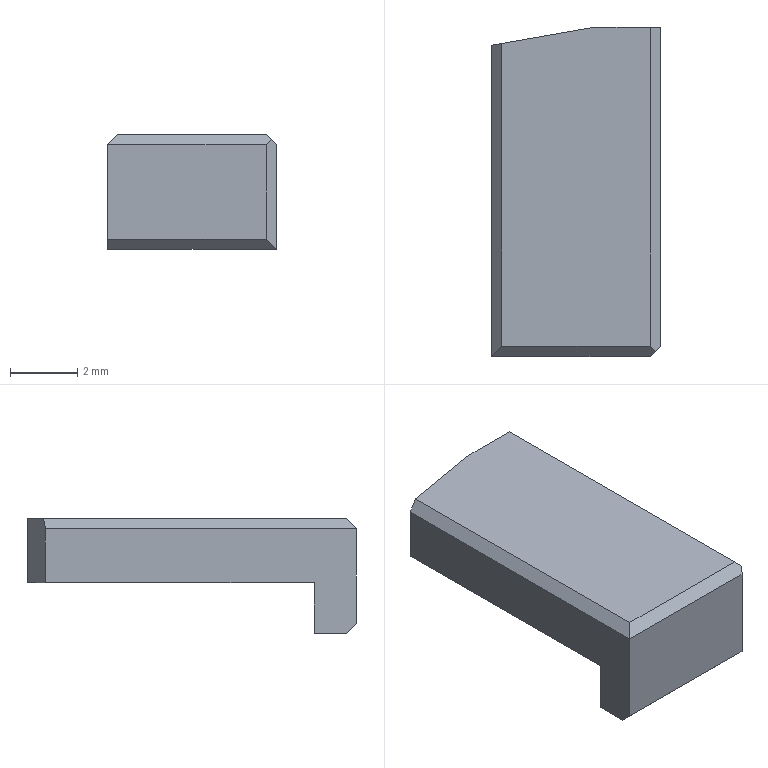Part | NX | 1 solid | 14 faces | box 5 x 9.75 x 3.4 mm | volume 99.073 mm3 | plane 14
STEP:
#1=CARTESIAN_POINT('',(-20.11,-56.129,7.853));
#2=VERTEX_POINT('',#1);
#3=CARTESIAN_POINT('',(-20.11,-64.629,7.853));
#4=VERTEX_POINT('',#3);
#5=CARTESIAN_POINT('',(-20.11,-63.129,7.853));
#6=DIRECTION('',(0.,-1.,0.));
#7=VECTOR('',#6,1000.);
#8=LINE('',#5,#7);
#9=EDGE_CURVE('',#2,#4,#8,.T.);
#10=ORIENTED_EDGE('',*,*,#9,.T.);
#11=CARTESIAN_POINT('',(-25.11,-64.629,7.853));
#12=VERTEX_POINT('',#11);
#13=CARTESIAN_POINT('',(-22.513,-64.629,7.853));
#14=DIRECTION('',(1.,0.,0.));
#15=VECTOR('',#14,1000.);
#16=LINE('',#13,#15);
#17=EDGE_CURVE('',#12,#4,#16,.T.);
#18=ORIENTED_EDGE('',*,*,#17,.F.);
#19=CARTESIAN_POINT('',(-25.11,-56.658,7.853));
#20=VERTEX_POINT('',#19);
#21=CARTESIAN_POINT('',(-25.11,-63.129,7.853));
#22=DIRECTION('',(0.,1.,0.));
#23=VECTOR('',#22,1000.);
#24=LINE('',#21,#23);
#25=EDGE_CURVE('',#12,#20,#24,.T.);
#26=ORIENTED_EDGE('',*,*,#25,.T.);
#27=CARTESIAN_POINT('',(-22.11,-56.129,7.853));
#28=VERTEX_POINT('',#27);
#29=CARTESIAN_POINT('',(-22.513,-56.2,7.853));
#30=DIRECTION('',(0.9848,0.1736,0.));
#31=VECTOR('',#30,1000.);
#32=LINE('',#29,#31);
#33=EDGE_CURVE('',#20,#28,#32,.T.);
#34=ORIENTED_EDGE('',*,*,#33,.T.);
#35=CARTESIAN_POINT('',(-22.513,-56.129,7.853));
#36=DIRECTION('',(1.,0.,0.));
#37=VECTOR('',#36,1000.);
#38=LINE('',#35,#37);
#39=EDGE_CURVE('',#28,#2,#38,.T.);
#40=ORIENTED_EDGE('',*,*,#39,.T.);
#41=EDGE_LOOP('',(#10,#18,#26,#34,#40));
#42=FACE_BOUND('',#41,.T.);
#43=CARTESIAN_POINT('',(-32.11,-63.129,7.853));
#44=DIRECTION('',(0.,0.,-1.));
#45=DIRECTION('',(0.,-1.,0.));
#46=AXIS2_PLACEMENT_3D('',#43,#44,#45);
#47=PLANE('',#46);
#48=ADVANCED_FACE('',(#42),#47,.T.);
#49=CARTESIAN_POINT('',(-25.11,-56.658,9.453));
#50=VERTEX_POINT('',#49);
#51=CARTESIAN_POINT('',(-25.11,-65.879,9.453));
#52=VERTEX_POINT('',#51);
#53=CARTESIAN_POINT('',(-25.11,-61.268,9.453));
#54=DIRECTION('',(0.,-1.,0.));
#55=VECTOR('',#54,1000.);
#56=LINE('',#53,#55);
#57=EDGE_CURVE('',#50,#52,#56,.T.);
#58=ORIENTED_EDGE('',*,*,#57,.F.);
#59=CARTESIAN_POINT('',(-25.11,-56.658,8.803));
#60=DIRECTION('',(0.,0.,-1.));
#61=VECTOR('',#60,1000.);
#62=LINE('',#59,#61);
#63=EDGE_CURVE('',#50,#20,#62,.T.);
#64=ORIENTED_EDGE('',*,*,#63,.T.);
#65=ORIENTED_EDGE('',*,*,#25,.F.);
#66=CARTESIAN_POINT('',(-25.11,-64.629,6.353));
#67=VERTEX_POINT('',#66);
#68=CARTESIAN_POINT('',(-25.11,-64.629,13.966));
#69=DIRECTION('',(0.,0.,-1.));
#70=VECTOR('',#69,1000.);
#71=LINE('',#68,#70);
#72=EDGE_CURVE('',#12,#67,#71,.T.);
#73=ORIENTED_EDGE('',*,*,#72,.T.);
#74=CARTESIAN_POINT('',(-25.11,-65.579,6.353));
#75=VERTEX_POINT('',#74);
#76=CARTESIAN_POINT('',(-25.11,-63.129,6.353));
#77=DIRECTION('',(0.,1.,0.));
#78=VECTOR('',#77,1000.);
#79=LINE('',#76,#78);
#80=EDGE_CURVE('',#75,#67,#79,.T.);
#81=ORIENTED_EDGE('',*,*,#80,.F.);
#82=CARTESIAN_POINT('',(-25.11,-65.879,6.653));
#83=VERTEX_POINT('',#82);
#84=CARTESIAN_POINT('',(-25.11,-63.129,3.903));
#85=DIRECTION('',(0.,0.7071,-0.7071));
#86=VECTOR('',#85,1000.);
#87=LINE('',#84,#86);
#88=EDGE_CURVE('',#83,#75,#87,.T.);
#89=ORIENTED_EDGE('',*,*,#88,.F.);
#90=CARTESIAN_POINT('',(-25.11,-65.879,13.966));
#91=DIRECTION('',(0.,0.,1.));
#92=VECTOR('',#91,1000.);
#93=LINE('',#90,#92);
#94=EDGE_CURVE('',#83,#52,#93,.T.);
#95=ORIENTED_EDGE('',*,*,#94,.T.);
#96=EDGE_LOOP('',(#58,#64,#65,#73,#81,#89,#95));
#97=FACE_BOUND('',#96,.T.);
#98=CARTESIAN_POINT('',(-25.11,-63.129,9.253));
#99=DIRECTION('',(-1.,0.,0.));
#100=DIRECTION('',(0.,0.,1.));
#101=AXIS2_PLACEMENT_3D('',#98,#99,#100);
#102=PLANE('',#101);
#103=ADVANCED_FACE('',(#97),#102,.T.);
#104=CARTESIAN_POINT('',(-20.41,-65.579,9.753));
#105=VERTEX_POINT('',#104);
#106=CARTESIAN_POINT('',(-20.41,-56.129,9.753));
#107=VERTEX_POINT('',#106);
#108=CARTESIAN_POINT('',(-20.41,-61.004,9.753));
#109=DIRECTION('',(0.,1.,0.));
#110=VECTOR('',#109,1000.);
#111=LINE('',#108,#110);
#112=EDGE_CURVE('',#105,#107,#111,.T.);
#113=ORIENTED_EDGE('',*,*,#112,.T.);
#114=CARTESIAN_POINT('',(-22.11,-56.129,9.753));
#115=VERTEX_POINT('',#114);
#116=CARTESIAN_POINT('',(-22.513,-56.129,9.753));
#117=DIRECTION('',(-1.,0.,0.));
#118=VECTOR('',#117,1000.);
#119=LINE('',#116,#118);
#120=EDGE_CURVE('',#107,#115,#119,.T.);
#121=ORIENTED_EDGE('',*,*,#120,.T.);
#122=CARTESIAN_POINT('',(-24.81,-56.605,9.753));
#123=VERTEX_POINT('',#122);
#124=CARTESIAN_POINT('',(-22.513,-56.2,9.753));
#125=DIRECTION('',(-0.9848,-0.1736,0.));
#126=VECTOR('',#125,1000.);
#127=LINE('',#124,#126);
#128=EDGE_CURVE('',#115,#123,#127,.T.);
#129=ORIENTED_EDGE('',*,*,#128,.T.);
#130=CARTESIAN_POINT('',(-24.81,-65.579,9.753));
#131=VERTEX_POINT('',#130);
#132=CARTESIAN_POINT('',(-24.81,-61.268,9.753));
#133=DIRECTION('',(0.,-1.,0.));
#134=VECTOR('',#133,1000.);
#135=LINE('',#132,#134);
#136=EDGE_CURVE('',#123,#131,#135,.T.);
#137=ORIENTED_EDGE('',*,*,#136,.T.);
#138=CARTESIAN_POINT('',(-22.61,-65.579,9.753));
#139=DIRECTION('',(1.,0.,0.));
#140=VECTOR('',#139,1000.);
#141=LINE('',#138,#140);
#142=EDGE_CURVE('',#131,#105,#141,.T.);
#143=ORIENTED_EDGE('',*,*,#142,.T.);
#144=EDGE_LOOP('',(#113,#121,#129,#137,#143));
#145=FACE_BOUND('',#144,.T.);
#146=CARTESIAN_POINT('',(-16.11,-63.129,9.753));
#147=DIRECTION('',(0.,0.,1.));
#148=DIRECTION('',(1.,0.,0.));
#149=AXIS2_PLACEMENT_3D('',#146,#147,#148);
#150=PLANE('',#149);
#151=ADVANCED_FACE('',(#145),#150,.T.);
#152=CARTESIAN_POINT('',(-20.11,-56.129,9.453));
#153=VERTEX_POINT('',#152);
#154=CARTESIAN_POINT('',(-20.11,-56.129,13.966));
#155=DIRECTION('',(0.,0.,1.));
#156=VECTOR('',#155,1000.);
#157=LINE('',#154,#156);
#158=EDGE_CURVE('',#2,#153,#157,.T.);
#159=ORIENTED_EDGE('',*,*,#158,.T.);
#160=CARTESIAN_POINT('',(-20.11,-65.579,9.453));
#161=VERTEX_POINT('',#160);
#162=CARTESIAN_POINT('',(-20.11,-61.004,9.453));
#163=DIRECTION('',(0.,1.,0.));
#164=VECTOR('',#163,1000.);
#165=LINE('',#162,#164);
#166=EDGE_CURVE('',#161,#153,#165,.T.);
#167=ORIENTED_EDGE('',*,*,#166,.F.);
#168=CARTESIAN_POINT('',(-20.11,-65.579,6.353));
#169=VERTEX_POINT('',#168);
#170=CARTESIAN_POINT('',(-20.11,-65.579,8.053));
#171=DIRECTION('',(0.,0.,1.));
#172=VECTOR('',#171,1000.);
#173=LINE('',#170,#172);
#174=EDGE_CURVE('',#169,#161,#173,.T.);
#175=ORIENTED_EDGE('',*,*,#174,.F.);
#176=CARTESIAN_POINT('',(-20.11,-64.629,6.353));
#177=VERTEX_POINT('',#176);
#178=CARTESIAN_POINT('',(-20.11,-63.129,6.353));
#179=DIRECTION('',(0.,-1.,0.));
#180=VECTOR('',#179,1000.);
#181=LINE('',#178,#180);
#182=EDGE_CURVE('',#177,#169,#181,.T.);
#183=ORIENTED_EDGE('',*,*,#182,.F.);
#184=CARTESIAN_POINT('',(-20.11,-64.629,13.966));
#185=DIRECTION('',(0.,0.,-1.));
#186=VECTOR('',#185,1000.);
#187=LINE('',#184,#186);
#188=EDGE_CURVE('',#4,#177,#187,.T.);
#189=ORIENTED_EDGE('',*,*,#188,.F.);
#190=ORIENTED_EDGE('',*,*,#9,.F.);
#191=EDGE_LOOP('',(#159,#167,#175,#183,#189,#190));
#192=FACE_BOUND('',#191,.T.);
#193=CARTESIAN_POINT('',(-20.11,-63.129,7.853));
#194=DIRECTION('',(1.,0.,0.));
#195=DIRECTION('',(0.,-1.,0.));
#196=AXIS2_PLACEMENT_3D('',#193,#194,#195);
#197=PLANE('',#196);
#198=ADVANCED_FACE('',(#192),#197,.T.);
#199=CARTESIAN_POINT('',(-22.61,-65.579,6.353));
#200=DIRECTION('',(-1.,0.,0.));
#201=VECTOR('',#200,1000.);
#202=LINE('',#199,#201);
#203=EDGE_CURVE('',#169,#75,#202,.T.);
#204=ORIENTED_EDGE('',*,*,#203,.T.);
#205=ORIENTED_EDGE('',*,*,#80,.T.);
#206=CARTESIAN_POINT('',(-22.513,-64.629,6.353));
#207=DIRECTION('',(1.,0.,0.));
#208=VECTOR('',#207,1000.);
#209=LINE('',#206,#208);
#210=EDGE_CURVE('',#67,#177,#209,.T.);
#211=ORIENTED_EDGE('',*,*,#210,.T.);
#212=ORIENTED_EDGE('',*,*,#182,.T.);
#213=EDGE_LOOP('',(#204,#205,#211,#212));
#214=FACE_BOUND('',#213,.T.);
#215=CARTESIAN_POINT('',(-19.282,-63.809,6.353));
#216=DIRECTION('',(0.,0.,-1.));
#217=DIRECTION('',(0.,-1.,0.));
#218=AXIS2_PLACEMENT_3D('',#215,#216,#217);
#219=PLANE('',#218);
#220=ADVANCED_FACE('',(#214),#219,.T.);
#221=ORIENTED_EDGE('',*,*,#57,.T.);
#222=CARTESIAN_POINT('',(-22.513,-63.282,12.05));
#223=DIRECTION('',(0.5774,0.5774,0.5774));
#224=VECTOR('',#223,1000.);
#225=LINE('',#222,#224);
#226=EDGE_CURVE('',#52,#131,#225,.T.);
#227=ORIENTED_EDGE('',*,*,#226,.T.);
#228=ORIENTED_EDGE('',*,*,#136,.F.);
#229=CARTESIAN_POINT('',(-22.513,-56.2,12.05));
#230=DIRECTION('',(-0.7017,-0.1237,-0.7017));
#231=VECTOR('',#230,1000.);
#232=LINE('',#229,#231);
#233=EDGE_CURVE('',#123,#50,#232,.T.);
#234=ORIENTED_EDGE('',*,*,#233,.T.);
#235=EDGE_LOOP('',(#221,#227,#228,#234));
#236=FACE_BOUND('',#235,.T.);
#237=CARTESIAN_POINT('',(-24.96,-61.268,9.603));
#238=DIRECTION('',(0.7071,0.,-0.7071));
#239=DIRECTION('',(0.,-1.,0.));
#240=AXIS2_PLACEMENT_3D('',#237,#238,#239);
#241=PLANE('',#240);
#242=ADVANCED_FACE('',(#236),#241,.F.);
#243=ORIENTED_EDGE('',*,*,#112,.F.);
#244=CARTESIAN_POINT('',(-20.26,-65.729,9.603));
#245=VERTEX_POINT('',#244);
#246=CARTESIAN_POINT('',(-22.86,-63.129,12.203));
#247=DIRECTION('',(-0.5774,0.5774,0.5774));
#248=VECTOR('',#247,1000.);
#249=LINE('',#246,#248);
#250=EDGE_CURVE('',#245,#105,#249,.T.);
#251=ORIENTED_EDGE('',*,*,#250,.F.);
#252=CARTESIAN_POINT('',(-17.66,-63.129,7.003));
#253=DIRECTION('',(0.5774,0.5774,-0.5774));
#254=VECTOR('',#253,1000.);
#255=LINE('',#252,#254);
#256=EDGE_CURVE('',#245,#161,#255,.T.);
#257=ORIENTED_EDGE('',*,*,#256,.T.);
#258=ORIENTED_EDGE('',*,*,#166,.T.);
#259=CARTESIAN_POINT('',(-24.624,-56.129,13.966));
#260=DIRECTION('',(0.7071,0.,-0.7071));
#261=VECTOR('',#260,1000.);
#262=LINE('',#259,#261);
#263=EDGE_CURVE('',#107,#153,#262,.T.);
#264=ORIENTED_EDGE('',*,*,#263,.F.);
#265=EDGE_LOOP('',(#243,#251,#257,#258,#264));
#266=FACE_BOUND('',#265,.T.);
#267=CARTESIAN_POINT('',(-20.26,-61.004,9.603));
#268=DIRECTION('',(0.7071,0.,0.7071));
#269=DIRECTION('',(0.,-1.,0.));
#270=AXIS2_PLACEMENT_3D('',#267,#268,#269);
#271=PLANE('',#270);
#272=ADVANCED_FACE('',(#266),#271,.T.);
#273=ORIENTED_EDGE('',*,*,#203,.F.);
#274=CARTESIAN_POINT('',(-20.41,-65.879,6.653));
#275=VERTEX_POINT('',#274);
#276=CARTESIAN_POINT('',(-17.66,-63.129,3.903));
#277=DIRECTION('',(0.5774,0.5774,-0.5774));
#278=VECTOR('',#277,1000.);
#279=LINE('',#276,#278);
#280=EDGE_CURVE('',#275,#169,#279,.T.);
#281=ORIENTED_EDGE('',*,*,#280,.F.);
#282=CARTESIAN_POINT('',(-22.61,-65.879,6.653));
#283=DIRECTION('',(-1.,0.,0.));
#284=VECTOR('',#283,1000.);
#285=LINE('',#282,#284);
#286=EDGE_CURVE('',#275,#83,#285,.T.);
#287=ORIENTED_EDGE('',*,*,#286,.T.);
#288=ORIENTED_EDGE('',*,*,#88,.T.);
#289=EDGE_LOOP('',(#273,#281,#287,#288));
#290=FACE_BOUND('',#289,.T.);
#291=CARTESIAN_POINT('',(-22.61,-65.729,6.503));
#292=DIRECTION('',(0.,-0.7071,-0.7071));
#293=DIRECTION('',(0.,-0.7071,0.7071));
#294=AXIS2_PLACEMENT_3D('',#291,#292,#293);
#295=PLANE('',#294);
#296=ADVANCED_FACE('',(#290),#295,.T.);
#297=CARTESIAN_POINT('',(-22.11,-56.129,8.803));
#298=DIRECTION('',(0.,0.,-1.));
#299=VECTOR('',#298,1000.);
#300=LINE('',#297,#299);
#301=EDGE_CURVE('',#115,#28,#300,.T.);
#302=ORIENTED_EDGE('',*,*,#301,.F.);
#303=ORIENTED_EDGE('',*,*,#120,.F.);
#304=ORIENTED_EDGE('',*,*,#263,.T.);
#305=ORIENTED_EDGE('',*,*,#158,.F.);
#306=ORIENTED_EDGE('',*,*,#39,.F.);
#307=EDGE_LOOP('',(#302,#303,#304,#305,#306));
#308=FACE_BOUND('',#307,.T.);
#309=CARTESIAN_POINT('',(-22.513,-56.129,13.966));
#310=DIRECTION('',(0.,-1.,0.));
#311=DIRECTION('',(-1.,0.,0.));
#312=AXIS2_PLACEMENT_3D('',#309,#310,#311);
#313=PLANE('',#312);
#314=ADVANCED_FACE('',(#308),#313,.F.);
#315=ORIENTED_EDGE('',*,*,#301,.T.);
#316=ORIENTED_EDGE('',*,*,#33,.F.);
#317=ORIENTED_EDGE('',*,*,#63,.F.);
#318=ORIENTED_EDGE('',*,*,#233,.F.);
#319=ORIENTED_EDGE('',*,*,#128,.F.);
#320=EDGE_LOOP('',(#315,#316,#317,#318,#319));
#321=FACE_BOUND('',#320,.T.);
#322=CARTESIAN_POINT('',(-23.61,-56.393,8.803));
#323=DIRECTION('',(0.1736,-0.9848,0.));
#324=DIRECTION('',(0.,0.,-1.));
#325=AXIS2_PLACEMENT_3D('',#322,#323,#324);
#326=PLANE('',#325);
#327=ADVANCED_FACE('',(#321),#326,.F.);
#328=CARTESIAN_POINT('',(-20.41,-65.879,9.453));
#329=VERTEX_POINT('',#328);
#330=CARTESIAN_POINT('',(-20.41,-65.879,8.053));
#331=DIRECTION('',(0.,0.,1.));
#332=VECTOR('',#331,1000.);
#333=LINE('',#330,#332);
#334=EDGE_CURVE('',#275,#329,#333,.T.);
#335=ORIENTED_EDGE('',*,*,#334,.T.);
#336=CARTESIAN_POINT('',(-22.61,-65.879,9.453));
#337=DIRECTION('',(1.,0.,0.));
#338=VECTOR('',#337,1000.);
#339=LINE('',#336,#338);
#340=EDGE_CURVE('',#52,#329,#339,.T.);
#341=ORIENTED_EDGE('',*,*,#340,.F.);
#342=ORIENTED_EDGE('',*,*,#94,.F.);
#343=ORIENTED_EDGE('',*,*,#286,.F.);
#344=EDGE_LOOP('',(#335,#341,#342,#343));
#345=FACE_BOUND('',#344,.T.);
#346=CARTESIAN_POINT('',(-20.513,-65.879,13.966));
#347=DIRECTION('',(0.,-1.,0.));
#348=DIRECTION('',(-1.,0.,0.));
#349=AXIS2_PLACEMENT_3D('',#346,#347,#348);
#350=PLANE('',#349);
#351=ADVANCED_FACE('',(#345),#350,.T.);
#352=ORIENTED_EDGE('',*,*,#17,.T.);
#353=ORIENTED_EDGE('',*,*,#188,.T.);
#354=ORIENTED_EDGE('',*,*,#210,.F.);
#355=ORIENTED_EDGE('',*,*,#72,.F.);
#356=EDGE_LOOP('',(#352,#353,#354,#355));
#357=FACE_BOUND('',#356,.T.);
#358=CARTESIAN_POINT('',(-16.21,-64.629,7.853));
#359=DIRECTION('',(0.,1.,0.));
#360=DIRECTION('',(1.,0.,0.));
#361=AXIS2_PLACEMENT_3D('',#358,#359,#360);
#362=PLANE('',#361);
#363=ADVANCED_FACE('',(#357),#362,.T.);
#364=ORIENTED_EDGE('',*,*,#340,.T.);
#365=CARTESIAN_POINT('',(-17.66,-63.129,12.203));
#366=DIRECTION('',(-0.5774,-0.5774,-0.5774));
#367=VECTOR('',#366,1000.);
#368=LINE('',#365,#367);
#369=EDGE_CURVE('',#245,#329,#368,.T.);
#370=ORIENTED_EDGE('',*,*,#369,.F.);
#371=ORIENTED_EDGE('',*,*,#250,.T.);
#372=ORIENTED_EDGE('',*,*,#142,.F.);
#373=ORIENTED_EDGE('',*,*,#226,.F.);
#374=EDGE_LOOP('',(#364,#370,#371,#372,#373));
#375=FACE_BOUND('',#374,.T.);
#376=CARTESIAN_POINT('',(-22.61,-65.729,9.603));
#377=DIRECTION('',(0.,0.7071,-0.7071));
#378=DIRECTION('',(-1.,0.,0.));
#379=AXIS2_PLACEMENT_3D('',#376,#377,#378);
#380=PLANE('',#379);
#381=ADVANCED_FACE('',(#375),#380,.F.);
#382=ORIENTED_EDGE('',*,*,#334,.F.);
#383=ORIENTED_EDGE('',*,*,#280,.T.);
#384=ORIENTED_EDGE('',*,*,#174,.T.);
#385=ORIENTED_EDGE('',*,*,#256,.F.);
#386=ORIENTED_EDGE('',*,*,#369,.T.);
#387=EDGE_LOOP('',(#382,#383,#384,#385,#386));
#388=FACE_BOUND('',#387,.T.);
#389=CARTESIAN_POINT('',(-20.26,-65.729,8.053));
#390=DIRECTION('',(0.7071,-0.7071,0.));
#391=DIRECTION('',(0.,0.,-1.));
#392=AXIS2_PLACEMENT_3D('',#389,#390,#391);
#393=PLANE('',#392);
#394=ADVANCED_FACE('',(#388),#393,.T.);
#395=CLOSED_SHELL('',(#48,#103,#151,#198,#220,#242,#272,#296,#314,#327,#351,#363,#381,#394));
#396=MANIFOLD_SOLID_BREP('',#395);
#397=(LENGTH_UNIT()NAMED_UNIT(*)SI_UNIT(.MILLI.,.METRE.));
#398=UNCERTAINTY_MEASURE_WITH_UNIT(LENGTH_MEASURE(0.00001),#397,'','');
#399=(NAMED_UNIT(*)PLANE_ANGLE_UNIT()SI_UNIT($,.RADIAN.));
#400=(NAMED_UNIT(*)SI_UNIT($,.STERADIAN.)SOLID_ANGLE_UNIT());
#401=(GEOMETRIC_REPRESENTATION_CONTEXT(3)GLOBAL_UNCERTAINTY_ASSIGNED_CONTEXT((#398))GLOBAL_UNIT_ASSIGNED_CONTEXT((#397,#399,#400))REPRESENTATION_CONTEXT('',''));
#402=ADVANCED_BREP_SHAPE_REPRESENTATION('',(#396),#401);